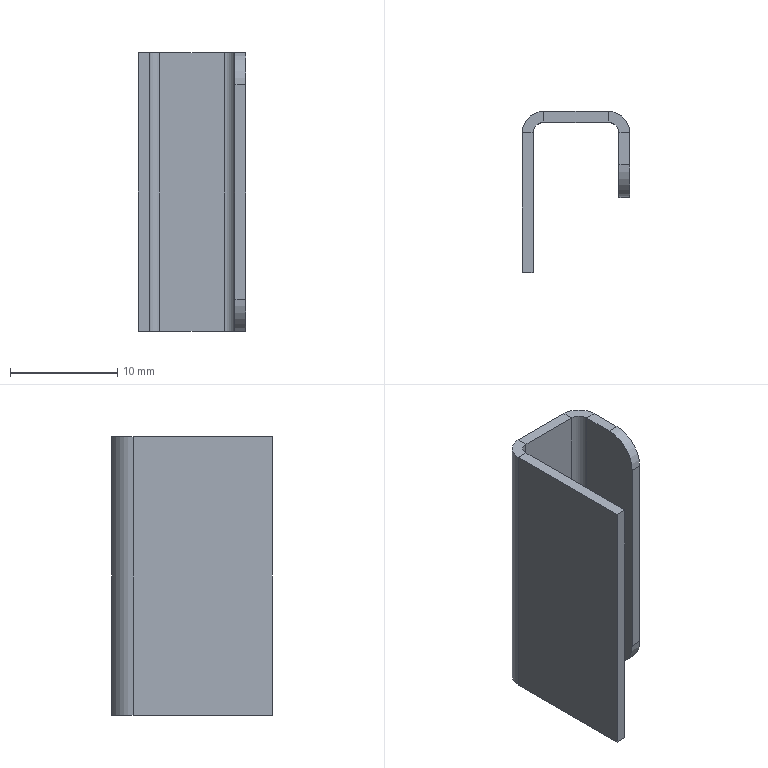Part | SolidWorks | features BaseBody 1 | 1 solid | 24 faces | box 10 x 15 x 26 mm | volume 768.659 mm3 | plane 18 | cylinder 6 | commonest cylinder face diameters 2 x2 4 x2 6 x2
STEP:
#1=CARTESIAN_POINT('',(10.,7.,-10.));
#2=VERTEX_POINT('',#1);
#3=CARTESIAN_POINT('',(10.,10.,-13.));
#4=VERTEX_POINT('',#3);
#5=CARTESIAN_POINT('',(10.,10.,-10.));
#6=DIRECTION('',(1.,0.,0.));
#7=DIRECTION('',(0.,-1.,0.));
#8=AXIS2_PLACEMENT_3D('',#5,#6,#7);
#9=CIRCLE('',#8,3.);
#10=EDGE_CURVE('',#2,#4,#9,.T.);
#11=ORIENTED_EDGE('',*,*,#10,.F.);
#12=CARTESIAN_POINT('',(9.,7.,-10.));
#13=VERTEX_POINT('',#12);
#14=CARTESIAN_POINT('',(10.,7.,-10.));
#15=DIRECTION('',(1.,0.,0.));
#16=VECTOR('',#15,1000.);
#17=LINE('',#14,#16);
#18=EDGE_CURVE('',#13,#2,#17,.T.);
#19=ORIENTED_EDGE('',*,*,#18,.F.);
#20=CARTESIAN_POINT('',(9.,10.,-13.));
#21=VERTEX_POINT('',#20);
#22=CARTESIAN_POINT('',(9.,10.,-10.));
#23=DIRECTION('',(-1.,0.,0.));
#24=DIRECTION('',(0.,-1.,0.));
#25=AXIS2_PLACEMENT_3D('',#22,#23,#24);
#26=CIRCLE('',#25,3.);
#27=EDGE_CURVE('',#21,#13,#26,.T.);
#28=ORIENTED_EDGE('',*,*,#27,.F.);
#29=CARTESIAN_POINT('',(8.,10.,-13.));
#30=DIRECTION('',(-1.,0.,0.));
#31=VECTOR('',#30,1000.);
#32=LINE('',#29,#31);
#33=EDGE_CURVE('',#4,#21,#32,.T.);
#34=ORIENTED_EDGE('',*,*,#33,.F.);
#35=EDGE_LOOP('',(#11,#19,#28,#34));
#36=FACE_OUTER_BOUND('',#35,.T.);
#37=CARTESIAN_POINT('',(8.,10.,-10.));
#38=DIRECTION('',(-1.,0.,0.));
#39=DIRECTION('',(0.,0.,1.));
#40=AXIS2_PLACEMENT_3D('',#37,#38,#39);
#41=CYLINDRICAL_SURFACE('',#40,3.);
#42=ADVANCED_FACE('',(#36),#41,.T.);
#43=CARTESIAN_POINT('',(10.,10.,13.));
#44=VERTEX_POINT('',#43);
#45=CARTESIAN_POINT('',(10.,7.,10.));
#46=VERTEX_POINT('',#45);
#47=CARTESIAN_POINT('',(10.,10.,10.));
#48=DIRECTION('',(1.,0.,0.));
#49=DIRECTION('',(0.,-1.,0.));
#50=AXIS2_PLACEMENT_3D('',#47,#48,#49);
#51=CIRCLE('',#50,3.);
#52=EDGE_CURVE('',#44,#46,#51,.T.);
#53=ORIENTED_EDGE('',*,*,#52,.F.);
#54=CARTESIAN_POINT('',(9.,10.,13.));
#55=VERTEX_POINT('',#54);
#56=CARTESIAN_POINT('',(10.,10.,13.));
#57=DIRECTION('',(1.,0.,0.));
#58=VECTOR('',#57,1000.);
#59=LINE('',#56,#58);
#60=EDGE_CURVE('',#55,#44,#59,.T.);
#61=ORIENTED_EDGE('',*,*,#60,.F.);
#62=CARTESIAN_POINT('',(9.,7.,10.));
#63=VERTEX_POINT('',#62);
#64=CARTESIAN_POINT('',(9.,10.,10.));
#65=DIRECTION('',(-1.,0.,0.));
#66=DIRECTION('',(0.,-1.,0.));
#67=AXIS2_PLACEMENT_3D('',#64,#65,#66);
#68=CIRCLE('',#67,3.);
#69=EDGE_CURVE('',#63,#55,#68,.T.);
#70=ORIENTED_EDGE('',*,*,#69,.F.);
#71=CARTESIAN_POINT('',(9.,7.,10.));
#72=DIRECTION('',(-1.,0.,0.));
#73=VECTOR('',#72,1000.);
#74=LINE('',#71,#73);
#75=EDGE_CURVE('',#46,#63,#74,.T.);
#76=ORIENTED_EDGE('',*,*,#75,.F.);
#77=EDGE_LOOP('',(#53,#61,#70,#76));
#78=FACE_OUTER_BOUND('',#77,.T.);
#79=CARTESIAN_POINT('',(10.,10.,10.));
#80=DIRECTION('',(1.,0.,0.));
#81=DIRECTION('',(0.,0.,-1.));
#82=AXIS2_PLACEMENT_3D('',#79,#80,#81);
#83=CYLINDRICAL_SURFACE('',#82,3.);
#84=ADVANCED_FACE('',(#78),#83,.T.);
#85=CARTESIAN_POINT('',(1.,0.,13.));
#86=VERTEX_POINT('',#85);
#87=CARTESIAN_POINT('',(1.,13.,13.));
#88=VERTEX_POINT('',#87);
#89=CARTESIAN_POINT('',(1.,0.,13.));
#90=DIRECTION('',(0.,1.,0.));
#91=VECTOR('',#90,1000.);
#92=LINE('',#89,#91);
#93=EDGE_CURVE('',#86,#88,#92,.T.);
#94=ORIENTED_EDGE('',*,*,#93,.T.);
#95=CARTESIAN_POINT('',(0.,13.,13.));
#96=VERTEX_POINT('',#95);
#97=CARTESIAN_POINT('',(1.,13.,13.));
#98=DIRECTION('',(-1.,0.,0.));
#99=VECTOR('',#98,1000.);
#100=LINE('',#97,#99);
#101=EDGE_CURVE('',#88,#96,#100,.T.);
#102=ORIENTED_EDGE('',*,*,#101,.T.);
#103=CARTESIAN_POINT('',(0.,0.,13.));
#104=VERTEX_POINT('',#103);
#105=CARTESIAN_POINT('',(0.,0.,13.));
#106=DIRECTION('',(0.,1.,0.));
#107=VECTOR('',#106,1000.);
#108=LINE('',#105,#107);
#109=EDGE_CURVE('',#104,#96,#108,.T.);
#110=ORIENTED_EDGE('',*,*,#109,.F.);
#111=CARTESIAN_POINT('',(1.,0.,13.));
#112=DIRECTION('',(-1.,0.,0.));
#113=VECTOR('',#112,1000.);
#114=LINE('',#111,#113);
#115=EDGE_CURVE('',#86,#104,#114,.T.);
#116=ORIENTED_EDGE('',*,*,#115,.F.);
#117=EDGE_LOOP('',(#94,#102,#110,#116));
#118=FACE_OUTER_BOUND('',#117,.T.);
#119=CARTESIAN_POINT('',(8.,13.,13.));
#120=DIRECTION('',(0.,0.,1.));
#121=DIRECTION('',(1.,0.,0.));
#122=AXIS2_PLACEMENT_3D('',#119,#120,#121);
#123=PLANE('',#122);
#124=ADVANCED_FACE('',(#118),#123,.T.);
#125=CARTESIAN_POINT('',(10.,13.,-13.));
#126=VERTEX_POINT('',#125);
#127=CARTESIAN_POINT('',(10.,15.,-13.));
#128=DIRECTION('',(0.,-1.,0.));
#129=VECTOR('',#128,1000.);
#130=LINE('',#127,#129);
#131=EDGE_CURVE('',#126,#4,#130,.T.);
#132=ORIENTED_EDGE('',*,*,#131,.T.);
#133=ORIENTED_EDGE('',*,*,#33,.T.);
#134=CARTESIAN_POINT('',(9.,13.,-13.));
#135=VERTEX_POINT('',#134);
#136=CARTESIAN_POINT('',(9.,15.,-13.));
#137=DIRECTION('',(0.,-1.,0.));
#138=VECTOR('',#137,1000.);
#139=LINE('',#136,#138);
#140=EDGE_CURVE('',#135,#21,#139,.T.);
#141=ORIENTED_EDGE('',*,*,#140,.F.);
#142=CARTESIAN_POINT('',(9.,13.,-13.));
#143=DIRECTION('',(1.,0.,0.));
#144=VECTOR('',#143,1000.);
#145=LINE('',#142,#144);
#146=EDGE_CURVE('',#135,#126,#145,.T.);
#147=ORIENTED_EDGE('',*,*,#146,.T.);
#148=EDGE_LOOP('',(#132,#133,#141,#147));
#149=FACE_OUTER_BOUND('',#148,.T.);
#150=CARTESIAN_POINT('',(8.,13.,-13.));
#151=DIRECTION('',(0.,0.,1.));
#152=DIRECTION('',(1.,0.,0.));
#153=AXIS2_PLACEMENT_3D('',#150,#151,#152);
#154=PLANE('',#153);
#155=ADVANCED_FACE('',(#149),#154,.F.);
#156=CARTESIAN_POINT('',(10.,7.,-13.));
#157=DIRECTION('',(0.,0.,1.));
#158=VECTOR('',#157,1000.);
#159=LINE('',#156,#158);
#160=EDGE_CURVE('',#2,#46,#159,.T.);
#161=ORIENTED_EDGE('',*,*,#160,.T.);
#162=ORIENTED_EDGE('',*,*,#75,.T.);
#163=CARTESIAN_POINT('',(9.,7.,-13.));
#164=DIRECTION('',(0.,0.,1.));
#165=VECTOR('',#164,1000.);
#166=LINE('',#163,#165);
#167=EDGE_CURVE('',#13,#63,#166,.T.);
#168=ORIENTED_EDGE('',*,*,#167,.F.);
#169=ORIENTED_EDGE('',*,*,#18,.T.);
#170=EDGE_LOOP('',(#161,#162,#168,#169));
#171=FACE_OUTER_BOUND('',#170,.T.);
#172=CARTESIAN_POINT('',(10.,7.,-13.));
#173=DIRECTION('',(0.,1.,0.));
#174=DIRECTION('',(1.,0.,0.));
#175=AXIS2_PLACEMENT_3D('',#172,#173,#174);
#176=PLANE('',#175);
#177=ADVANCED_FACE('',(#171),#176,.F.);
#178=CARTESIAN_POINT('',(10.,13.,13.));
#179=VERTEX_POINT('',#178);
#180=CARTESIAN_POINT('',(10.,15.,13.));
#181=DIRECTION('',(0.,-1.,0.));
#182=VECTOR('',#181,1000.);
#183=LINE('',#180,#182);
#184=EDGE_CURVE('',#179,#44,#183,.T.);
#185=ORIENTED_EDGE('',*,*,#184,.T.);
#186=ORIENTED_EDGE('',*,*,#52,.T.);
#187=ORIENTED_EDGE('',*,*,#160,.F.);
#188=ORIENTED_EDGE('',*,*,#10,.T.);
#189=ORIENTED_EDGE('',*,*,#131,.F.);
#190=CARTESIAN_POINT('',(10.,13.,-13.));
#191=DIRECTION('',(0.,0.,1.));
#192=VECTOR('',#191,1000.);
#193=LINE('',#190,#192);
#194=EDGE_CURVE('',#126,#179,#193,.T.);
#195=ORIENTED_EDGE('',*,*,#194,.T.);
#196=EDGE_LOOP('',(#185,#186,#187,#188,#189,#195));
#197=FACE_OUTER_BOUND('',#196,.T.);
#198=CARTESIAN_POINT('',(10.,15.,-13.));
#199=DIRECTION('',(-1.,0.,0.));
#200=DIRECTION('',(0.,1.,0.));
#201=AXIS2_PLACEMENT_3D('',#198,#199,#200);
#202=PLANE('',#201);
#203=ADVANCED_FACE('',(#197),#202,.F.);
#204=CARTESIAN_POINT('',(8.,15.,13.));
#205=VERTEX_POINT('',#204);
#206=CARTESIAN_POINT('',(8.,13.,13.));
#207=DIRECTION('',(0.,0.,-1.));
#208=DIRECTION('',(1.,0.,0.));
#209=AXIS2_PLACEMENT_3D('',#206,#207,#208);
#210=CIRCLE('',#209,2.);
#211=EDGE_CURVE('',#205,#179,#210,.T.);
#212=ORIENTED_EDGE('',*,*,#211,.T.);
#213=ORIENTED_EDGE('',*,*,#194,.F.);
#214=CARTESIAN_POINT('',(8.,15.,-13.));
#215=VERTEX_POINT('',#214);
#216=CARTESIAN_POINT('',(8.,13.,-13.));
#217=DIRECTION('',(0.,0.,-1.));
#218=DIRECTION('',(1.,0.,0.));
#219=AXIS2_PLACEMENT_3D('',#216,#217,#218);
#220=CIRCLE('',#219,2.);
#221=EDGE_CURVE('',#215,#126,#220,.T.);
#222=ORIENTED_EDGE('',*,*,#221,.F.);
#223=CARTESIAN_POINT('',(8.,15.,-13.));
#224=DIRECTION('',(0.,0.,1.));
#225=VECTOR('',#224,1000.);
#226=LINE('',#223,#225);
#227=EDGE_CURVE('',#215,#205,#226,.T.);
#228=ORIENTED_EDGE('',*,*,#227,.T.);
#229=EDGE_LOOP('',(#212,#213,#222,#228));
#230=FACE_OUTER_BOUND('',#229,.T.);
#231=CARTESIAN_POINT('',(8.,13.,-13.));
#232=DIRECTION('',(0.,0.,1.));
#233=DIRECTION('',(1.,0.,0.));
#234=AXIS2_PLACEMENT_3D('',#231,#232,#233);
#235=CYLINDRICAL_SURFACE('',#234,2.);
#236=ADVANCED_FACE('',(#230),#235,.T.);
#237=CARTESIAN_POINT('',(2.,15.,13.));
#238=VERTEX_POINT('',#237);
#239=CARTESIAN_POINT('',(0.,15.,13.));
#240=DIRECTION('',(1.,0.,0.));
#241=VECTOR('',#240,1000.);
#242=LINE('',#239,#241);
#243=EDGE_CURVE('',#238,#205,#242,.T.);
#244=ORIENTED_EDGE('',*,*,#243,.T.);
#245=ORIENTED_EDGE('',*,*,#227,.F.);
#246=CARTESIAN_POINT('',(2.,15.,-13.));
#247=VERTEX_POINT('',#246);
#248=CARTESIAN_POINT('',(0.,15.,-13.));
#249=DIRECTION('',(1.,0.,0.));
#250=VECTOR('',#249,1000.);
#251=LINE('',#248,#250);
#252=EDGE_CURVE('',#247,#215,#251,.T.);
#253=ORIENTED_EDGE('',*,*,#252,.F.);
#254=CARTESIAN_POINT('',(2.,15.,-13.));
#255=DIRECTION('',(0.,0.,1.));
#256=VECTOR('',#255,1000.);
#257=LINE('',#254,#256);
#258=EDGE_CURVE('',#247,#238,#257,.T.);
#259=ORIENTED_EDGE('',*,*,#258,.T.);
#260=EDGE_LOOP('',(#244,#245,#253,#259));
#261=FACE_OUTER_BOUND('',#260,.T.);
#262=CARTESIAN_POINT('',(0.,15.,-13.));
#263=DIRECTION('',(0.,-1.,0.));
#264=DIRECTION('',(-1.,0.,0.));
#265=AXIS2_PLACEMENT_3D('',#262,#263,#264);
#266=PLANE('',#265);
#267=ADVANCED_FACE('',(#261),#266,.F.);
#268=CARTESIAN_POINT('',(2.,13.,13.));
#269=DIRECTION('',(0.,0.,-1.));
#270=DIRECTION('',(1.,0.,0.));
#271=AXIS2_PLACEMENT_3D('',#268,#269,#270);
#272=CIRCLE('',#271,2.);
#273=EDGE_CURVE('',#96,#238,#272,.T.);
#274=ORIENTED_EDGE('',*,*,#273,.T.);
#275=ORIENTED_EDGE('',*,*,#258,.F.);
#276=CARTESIAN_POINT('',(0.,13.,-13.));
#277=VERTEX_POINT('',#276);
#278=CARTESIAN_POINT('',(2.,13.,-13.));
#279=DIRECTION('',(0.,0.,-1.));
#280=DIRECTION('',(1.,0.,0.));
#281=AXIS2_PLACEMENT_3D('',#278,#279,#280);
#282=CIRCLE('',#281,2.);
#283=EDGE_CURVE('',#277,#247,#282,.T.);
#284=ORIENTED_EDGE('',*,*,#283,.F.);
#285=CARTESIAN_POINT('',(0.,13.,-13.));
#286=DIRECTION('',(0.,0.,1.));
#287=VECTOR('',#286,1000.);
#288=LINE('',#285,#287);
#289=EDGE_CURVE('',#277,#96,#288,.T.);
#290=ORIENTED_EDGE('',*,*,#289,.T.);
#291=EDGE_LOOP('',(#274,#275,#284,#290));
#292=FACE_OUTER_BOUND('',#291,.T.);
#293=CARTESIAN_POINT('',(2.,13.,-13.));
#294=DIRECTION('',(0.,0.,1.));
#295=DIRECTION('',(1.,0.,0.));
#296=AXIS2_PLACEMENT_3D('',#293,#294,#295);
#297=CYLINDRICAL_SURFACE('',#296,2.);
#298=ADVANCED_FACE('',(#292),#297,.T.);
#299=ORIENTED_EDGE('',*,*,#109,.T.);
#300=ORIENTED_EDGE('',*,*,#289,.F.);
#301=CARTESIAN_POINT('',(0.,0.,-13.));
#302=VERTEX_POINT('',#301);
#303=CARTESIAN_POINT('',(0.,0.,-13.));
#304=DIRECTION('',(0.,1.,0.));
#305=VECTOR('',#304,1000.);
#306=LINE('',#303,#305);
#307=EDGE_CURVE('',#302,#277,#306,.T.);
#308=ORIENTED_EDGE('',*,*,#307,.F.);
#309=CARTESIAN_POINT('',(0.,0.,-13.));
#310=DIRECTION('',(0.,0.,1.));
#311=VECTOR('',#310,1000.);
#312=LINE('',#309,#311);
#313=EDGE_CURVE('',#302,#104,#312,.T.);
#314=ORIENTED_EDGE('',*,*,#313,.T.);
#315=EDGE_LOOP('',(#299,#300,#308,#314));
#316=FACE_OUTER_BOUND('',#315,.T.);
#317=CARTESIAN_POINT('',(0.,0.,-13.));
#318=DIRECTION('',(1.,0.,0.));
#319=DIRECTION('',(0.,0.,-1.));
#320=AXIS2_PLACEMENT_3D('',#317,#318,#319);
#321=PLANE('',#320);
#322=ADVANCED_FACE('',(#316),#321,.F.);
#323=ORIENTED_EDGE('',*,*,#115,.T.);
#324=ORIENTED_EDGE('',*,*,#313,.F.);
#325=CARTESIAN_POINT('',(1.,0.,-13.));
#326=VERTEX_POINT('',#325);
#327=CARTESIAN_POINT('',(1.,0.,-13.));
#328=DIRECTION('',(-1.,0.,0.));
#329=VECTOR('',#328,1000.);
#330=LINE('',#327,#329);
#331=EDGE_CURVE('',#326,#302,#330,.T.);
#332=ORIENTED_EDGE('',*,*,#331,.F.);
#333=CARTESIAN_POINT('',(1.,0.,-13.));
#334=DIRECTION('',(0.,0.,1.));
#335=VECTOR('',#334,1000.);
#336=LINE('',#333,#335);
#337=EDGE_CURVE('',#326,#86,#336,.T.);
#338=ORIENTED_EDGE('',*,*,#337,.T.);
#339=EDGE_LOOP('',(#323,#324,#332,#338));
#340=FACE_OUTER_BOUND('',#339,.T.);
#341=CARTESIAN_POINT('',(1.,0.,-13.));
#342=DIRECTION('',(0.,1.,0.));
#343=DIRECTION('',(1.,0.,0.));
#344=AXIS2_PLACEMENT_3D('',#341,#342,#343);
#345=PLANE('',#344);
#346=ADVANCED_FACE('',(#340),#345,.F.);
#347=ORIENTED_EDGE('',*,*,#93,.F.);
#348=ORIENTED_EDGE('',*,*,#337,.F.);
#349=CARTESIAN_POINT('',(1.,13.,-13.));
#350=VERTEX_POINT('',#349);
#351=CARTESIAN_POINT('',(1.,0.,-13.));
#352=DIRECTION('',(0.,1.,0.));
#353=VECTOR('',#352,1000.);
#354=LINE('',#351,#353);
#355=EDGE_CURVE('',#326,#350,#354,.T.);
#356=ORIENTED_EDGE('',*,*,#355,.T.);
#357=CARTESIAN_POINT('',(1.,13.,-13.));
#358=DIRECTION('',(0.,0.,1.));
#359=VECTOR('',#358,1000.);
#360=LINE('',#357,#359);
#361=EDGE_CURVE('',#350,#88,#360,.T.);
#362=ORIENTED_EDGE('',*,*,#361,.T.);
#363=EDGE_LOOP('',(#347,#348,#356,#362));
#364=FACE_OUTER_BOUND('',#363,.T.);
#365=CARTESIAN_POINT('',(1.,0.,-13.));
#366=DIRECTION('',(1.,0.,0.));
#367=DIRECTION('',(0.,0.,-1.));
#368=AXIS2_PLACEMENT_3D('',#365,#366,#367);
#369=PLANE('',#368);
#370=ADVANCED_FACE('',(#364),#369,.T.);
#371=CARTESIAN_POINT('',(2.,14.,13.));
#372=VERTEX_POINT('',#371);
#373=CARTESIAN_POINT('',(2.,13.,13.));
#374=DIRECTION('',(0.,0.,-1.));
#375=DIRECTION('',(1.,0.,0.));
#376=AXIS2_PLACEMENT_3D('',#373,#374,#375);
#377=CIRCLE('',#376,1.);
#378=EDGE_CURVE('',#88,#372,#377,.T.);
#379=ORIENTED_EDGE('',*,*,#378,.F.);
#380=ORIENTED_EDGE('',*,*,#361,.F.);
#381=CARTESIAN_POINT('',(2.,14.,-13.));
#382=VERTEX_POINT('',#381);
#383=CARTESIAN_POINT('',(2.,13.,-13.));
#384=DIRECTION('',(0.,0.,-1.));
#385=DIRECTION('',(1.,0.,0.));
#386=AXIS2_PLACEMENT_3D('',#383,#384,#385);
#387=CIRCLE('',#386,1.);
#388=EDGE_CURVE('',#350,#382,#387,.T.);
#389=ORIENTED_EDGE('',*,*,#388,.T.);
#390=CARTESIAN_POINT('',(2.,14.,-13.));
#391=DIRECTION('',(0.,0.,1.));
#392=VECTOR('',#391,1000.);
#393=LINE('',#390,#392);
#394=EDGE_CURVE('',#382,#372,#393,.T.);
#395=ORIENTED_EDGE('',*,*,#394,.T.);
#396=EDGE_LOOP('',(#379,#380,#389,#395));
#397=FACE_OUTER_BOUND('',#396,.T.);
#398=CARTESIAN_POINT('',(2.,13.,-13.));
#399=DIRECTION('',(0.,0.,1.));
#400=DIRECTION('',(1.,0.,0.));
#401=AXIS2_PLACEMENT_3D('',#398,#399,#400);
#402=CYLINDRICAL_SURFACE('',#401,1.);
#403=ADVANCED_FACE('',(#397),#402,.F.);
#404=CARTESIAN_POINT('',(8.,14.,13.));
#405=VERTEX_POINT('',#404);
#406=CARTESIAN_POINT('',(0.,14.,13.));
#407=DIRECTION('',(1.,0.,0.));
#408=VECTOR('',#407,1000.);
#409=LINE('',#406,#408);
#410=EDGE_CURVE('',#372,#405,#409,.T.);
#411=ORIENTED_EDGE('',*,*,#410,.F.);
#412=ORIENTED_EDGE('',*,*,#394,.F.);
#413=CARTESIAN_POINT('',(8.,14.,-13.));
#414=VERTEX_POINT('',#413);
#415=CARTESIAN_POINT('',(0.,14.,-13.));
#416=DIRECTION('',(1.,0.,0.));
#417=VECTOR('',#416,1000.);
#418=LINE('',#415,#417);
#419=EDGE_CURVE('',#382,#414,#418,.T.);
#420=ORIENTED_EDGE('',*,*,#419,.T.);
#421=CARTESIAN_POINT('',(8.,14.,-13.));
#422=DIRECTION('',(0.,0.,1.));
#423=VECTOR('',#422,1000.);
#424=LINE('',#421,#423);
#425=EDGE_CURVE('',#414,#405,#424,.T.);
#426=ORIENTED_EDGE('',*,*,#425,.T.);
#427=EDGE_LOOP('',(#411,#412,#420,#426));
#428=FACE_OUTER_BOUND('',#427,.T.);
#429=CARTESIAN_POINT('',(0.,14.,-13.));
#430=DIRECTION('',(0.,-1.,0.));
#431=DIRECTION('',(-1.,0.,0.));
#432=AXIS2_PLACEMENT_3D('',#429,#430,#431);
#433=PLANE('',#432);
#434=ADVANCED_FACE('',(#428),#433,.T.);
#435=CARTESIAN_POINT('',(9.,13.,13.));
#436=VERTEX_POINT('',#435);
#437=CARTESIAN_POINT('',(8.,13.,13.));
#438=DIRECTION('',(0.,0.,-1.));
#439=DIRECTION('',(1.,0.,0.));
#440=AXIS2_PLACEMENT_3D('',#437,#438,#439);
#441=CIRCLE('',#440,1.);
#442=EDGE_CURVE('',#405,#436,#441,.T.);
#443=ORIENTED_EDGE('',*,*,#442,.F.);
#444=ORIENTED_EDGE('',*,*,#425,.F.);
#445=CARTESIAN_POINT('',(8.,13.,-13.));
#446=DIRECTION('',(0.,0.,-1.));
#447=DIRECTION('',(1.,0.,0.));
#448=AXIS2_PLACEMENT_3D('',#445,#446,#447);
#449=CIRCLE('',#448,1.);
#450=EDGE_CURVE('',#414,#135,#449,.T.);
#451=ORIENTED_EDGE('',*,*,#450,.T.);
#452=CARTESIAN_POINT('',(9.,13.,-13.));
#453=DIRECTION('',(0.,0.,1.));
#454=VECTOR('',#453,1000.);
#455=LINE('',#452,#454);
#456=EDGE_CURVE('',#135,#436,#455,.T.);
#457=ORIENTED_EDGE('',*,*,#456,.T.);
#458=EDGE_LOOP('',(#443,#444,#451,#457));
#459=FACE_OUTER_BOUND('',#458,.T.);
#460=CARTESIAN_POINT('',(8.,13.,-13.));
#461=DIRECTION('',(0.,0.,1.));
#462=DIRECTION('',(1.,0.,0.));
#463=AXIS2_PLACEMENT_3D('',#460,#461,#462);
#464=CYLINDRICAL_SURFACE('',#463,1.);
#465=ADVANCED_FACE('',(#459),#464,.F.);
#466=ORIENTED_EDGE('',*,*,#167,.T.);
#467=ORIENTED_EDGE('',*,*,#69,.T.);
#468=CARTESIAN_POINT('',(9.,15.,13.));
#469=DIRECTION('',(0.,-1.,0.));
#470=VECTOR('',#469,1000.);
#471=LINE('',#468,#470);
#472=EDGE_CURVE('',#436,#55,#471,.T.);
#473=ORIENTED_EDGE('',*,*,#472,.F.);
#474=ORIENTED_EDGE('',*,*,#456,.F.);
#475=ORIENTED_EDGE('',*,*,#140,.T.);
#476=ORIENTED_EDGE('',*,*,#27,.T.);
#477=EDGE_LOOP('',(#466,#467,#473,#474,#475,#476));
#478=FACE_OUTER_BOUND('',#477,.T.);
#479=CARTESIAN_POINT('',(9.,15.,-13.));
#480=DIRECTION('',(-1.,0.,0.));
#481=DIRECTION('',(0.,1.,0.));
#482=AXIS2_PLACEMENT_3D('',#479,#480,#481);
#483=PLANE('',#482);
#484=ADVANCED_FACE('',(#478),#483,.T.);
#485=ORIENTED_EDGE('',*,*,#472,.T.);
#486=ORIENTED_EDGE('',*,*,#60,.T.);
#487=ORIENTED_EDGE('',*,*,#184,.F.);
#488=CARTESIAN_POINT('',(10.,13.,13.));
#489=DIRECTION('',(-1.,0.,0.));
#490=VECTOR('',#489,1000.);
#491=LINE('',#488,#490);
#492=EDGE_CURVE('',#179,#436,#491,.T.);
#493=ORIENTED_EDGE('',*,*,#492,.T.);
#494=EDGE_LOOP('',(#485,#486,#487,#493));
#495=FACE_OUTER_BOUND('',#494,.T.);
#496=CARTESIAN_POINT('',(8.,14.,13.));
#497=DIRECTION('',(0.,0.,1.));
#498=DIRECTION('',(1.,0.,0.));
#499=AXIS2_PLACEMENT_3D('',#496,#497,#498);
#500=PLANE('',#499);
#501=ADVANCED_FACE('',(#495),#500,.T.);
#502=ORIENTED_EDGE('',*,*,#492,.F.);
#503=ORIENTED_EDGE('',*,*,#211,.F.);
#504=CARTESIAN_POINT('',(8.,14.,13.));
#505=DIRECTION('',(0.,1.,0.));
#506=VECTOR('',#505,1000.);
#507=LINE('',#504,#506);
#508=EDGE_CURVE('',#405,#205,#507,.T.);
#509=ORIENTED_EDGE('',*,*,#508,.F.);
#510=ORIENTED_EDGE('',*,*,#442,.T.);
#511=EDGE_LOOP('',(#502,#503,#509,#510));
#512=FACE_OUTER_BOUND('',#511,.T.);
#513=CARTESIAN_POINT('',(10.,13.,13.));
#514=DIRECTION('',(0.,0.,1.));
#515=DIRECTION('',(1.,0.,0.));
#516=AXIS2_PLACEMENT_3D('',#513,#514,#515);
#517=PLANE('',#516);
#518=ADVANCED_FACE('',(#512),#517,.T.);
#519=ORIENTED_EDGE('',*,*,#252,.T.);
#520=CARTESIAN_POINT('',(8.,15.,-13.));
#521=DIRECTION('',(0.,-1.,0.));
#522=VECTOR('',#521,1000.);
#523=LINE('',#520,#522);
#524=EDGE_CURVE('',#215,#414,#523,.T.);
#525=ORIENTED_EDGE('',*,*,#524,.T.);
#526=ORIENTED_EDGE('',*,*,#419,.F.);
#527=CARTESIAN_POINT('',(2.,14.,-13.));
#528=DIRECTION('',(0.,1.,0.));
#529=VECTOR('',#528,1000.);
#530=LINE('',#527,#529);
#531=EDGE_CURVE('',#382,#247,#530,.T.);
#532=ORIENTED_EDGE('',*,*,#531,.T.);
#533=EDGE_LOOP('',(#519,#525,#526,#532));
#534=FACE_OUTER_BOUND('',#533,.T.);
#535=CARTESIAN_POINT('',(9.,13.,-13.));
#536=DIRECTION('',(0.,0.,-1.));
#537=DIRECTION('',(0.,-1.,0.));
#538=AXIS2_PLACEMENT_3D('',#535,#536,#537);
#539=PLANE('',#538);
#540=ADVANCED_FACE('',(#534),#539,.T.);
#541=ORIENTED_EDGE('',*,*,#524,.F.);
#542=ORIENTED_EDGE('',*,*,#221,.T.);
#543=ORIENTED_EDGE('',*,*,#146,.F.);
#544=ORIENTED_EDGE('',*,*,#450,.F.);
#545=EDGE_LOOP('',(#541,#542,#543,#544));
#546=FACE_OUTER_BOUND('',#545,.T.);
#547=CARTESIAN_POINT('',(8.,15.,-13.));
#548=DIRECTION('',(0.,0.,-1.));
#549=DIRECTION('',(0.,-1.,0.));
#550=AXIS2_PLACEMENT_3D('',#547,#548,#549);
#551=PLANE('',#550);
#552=ADVANCED_FACE('',(#546),#551,.T.);
#553=ORIENTED_EDGE('',*,*,#243,.F.);
#554=CARTESIAN_POINT('',(2.,15.,13.));
#555=DIRECTION('',(0.,-1.,0.));
#556=VECTOR('',#555,1000.);
#557=LINE('',#554,#556);
#558=EDGE_CURVE('',#238,#372,#557,.T.);
#559=ORIENTED_EDGE('',*,*,#558,.T.);
#560=ORIENTED_EDGE('',*,*,#410,.T.);
#561=ORIENTED_EDGE('',*,*,#508,.T.);
#562=EDGE_LOOP('',(#553,#559,#560,#561));
#563=FACE_OUTER_BOUND('',#562,.T.);
#564=CARTESIAN_POINT('',(1.,13.,13.));
#565=DIRECTION('',(0.,0.,1.));
#566=DIRECTION('',(1.,0.,0.));
#567=AXIS2_PLACEMENT_3D('',#564,#565,#566);
#568=PLANE('',#567);
#569=ADVANCED_FACE('',(#563),#568,.T.);
#570=ORIENTED_EDGE('',*,*,#558,.F.);
#571=ORIENTED_EDGE('',*,*,#273,.F.);
#572=ORIENTED_EDGE('',*,*,#101,.F.);
#573=ORIENTED_EDGE('',*,*,#378,.T.);
#574=EDGE_LOOP('',(#570,#571,#572,#573));
#575=FACE_OUTER_BOUND('',#574,.T.);
#576=CARTESIAN_POINT('',(2.,15.,13.));
#577=DIRECTION('',(0.,0.,1.));
#578=DIRECTION('',(1.,0.,0.));
#579=AXIS2_PLACEMENT_3D('',#576,#577,#578);
#580=PLANE('',#579);
#581=ADVANCED_FACE('',(#575),#580,.T.);
#582=ORIENTED_EDGE('',*,*,#307,.T.);
#583=CARTESIAN_POINT('',(0.,13.,-13.));
#584=DIRECTION('',(1.,0.,0.));
#585=VECTOR('',#584,1000.);
#586=LINE('',#583,#585);
#587=EDGE_CURVE('',#277,#350,#586,.T.);
#588=ORIENTED_EDGE('',*,*,#587,.T.);
#589=ORIENTED_EDGE('',*,*,#355,.F.);
#590=ORIENTED_EDGE('',*,*,#331,.T.);
#591=EDGE_LOOP('',(#582,#588,#589,#590));
#592=FACE_OUTER_BOUND('',#591,.T.);
#593=CARTESIAN_POINT('',(2.,14.,-13.));
#594=DIRECTION('',(0.,0.,-1.));
#595=DIRECTION('',(0.,-1.,0.));
#596=AXIS2_PLACEMENT_3D('',#593,#594,#595);
#597=PLANE('',#596);
#598=ADVANCED_FACE('',(#592),#597,.T.);
#599=ORIENTED_EDGE('',*,*,#587,.F.);
#600=ORIENTED_EDGE('',*,*,#283,.T.);
#601=ORIENTED_EDGE('',*,*,#531,.F.);
#602=ORIENTED_EDGE('',*,*,#388,.F.);
#603=EDGE_LOOP('',(#599,#600,#601,#602));
#604=FACE_OUTER_BOUND('',#603,.T.);
#605=CARTESIAN_POINT('',(0.,13.,-13.));
#606=DIRECTION('',(0.,0.,-1.));
#607=DIRECTION('',(0.,-1.,0.));
#608=AXIS2_PLACEMENT_3D('',#605,#606,#607);
#609=PLANE('',#608);
#610=ADVANCED_FACE('',(#604),#609,.T.);
#611=CLOSED_SHELL('',(#42,#84,#124,#155,#177,#203,#236,#267,#298,#322,#346,#370,#403,#434,#465,#484,#501,#518,#540,#552,#569,#581,#598,#610));
#612=MANIFOLD_SOLID_BREP('',#611);
#613=CARTESIAN_POINT('',(0.,0.,0.));
#614=DIRECTION('',(0.,0.,1.));
#615=DIRECTION('',(1.,0.,0.));
#616=AXIS2_PLACEMENT_3D('',#613,#614,#615);
#617=(LENGTH_UNIT()NAMED_UNIT(*)SI_UNIT(.MILLI.,.METRE.));
#618=UNCERTAINTY_MEASURE_WITH_UNIT(LENGTH_MEASURE(0.00001),#617,'','');
#619=(NAMED_UNIT(*)PLANE_ANGLE_UNIT()SI_UNIT($,.RADIAN.));
#620=(NAMED_UNIT(*)SI_UNIT($,.STERADIAN.)SOLID_ANGLE_UNIT());
#621=(GEOMETRIC_REPRESENTATION_CONTEXT(3)GLOBAL_UNCERTAINTY_ASSIGNED_CONTEXT((#618))GLOBAL_UNIT_ASSIGNED_CONTEXT((#617,#619,#620))REPRESENTATION_CONTEXT('',''));
#622=ADVANCED_BREP_SHAPE_REPRESENTATION('',(#612,#616),#621);